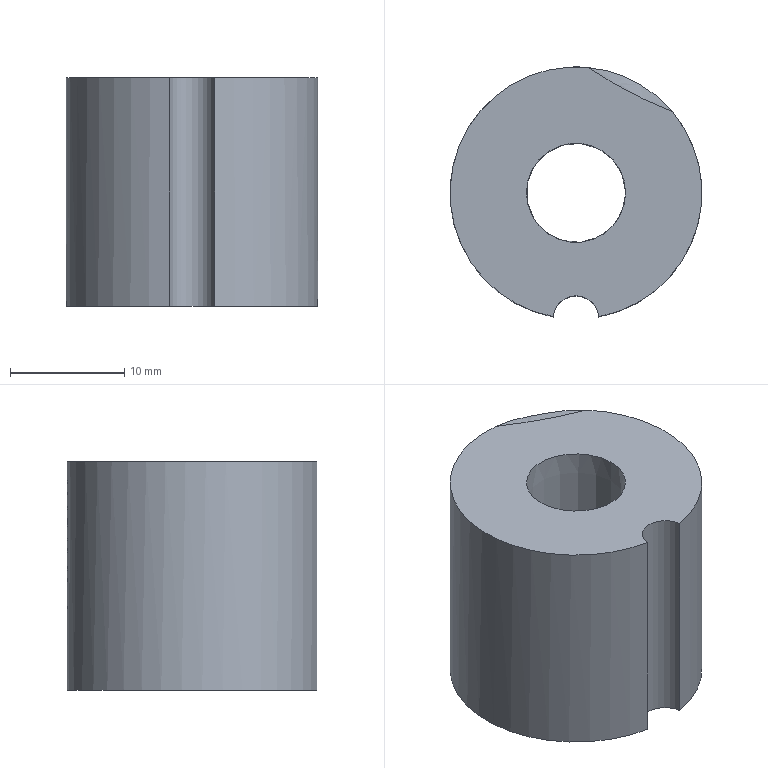Part | NX | features EKSD22-20-P8.66_2 2 | 1 solid | 205 faces | box 22 x 21.818 x 20 mm | volume 4998 mm3 | plane 111 | cylinder 92 | cone 1 | spline 1 | commonest cylinder face diameters 21.8 x15 22 x8 0.533 x3 0.805 x3 0.811 x3 0.869 x3